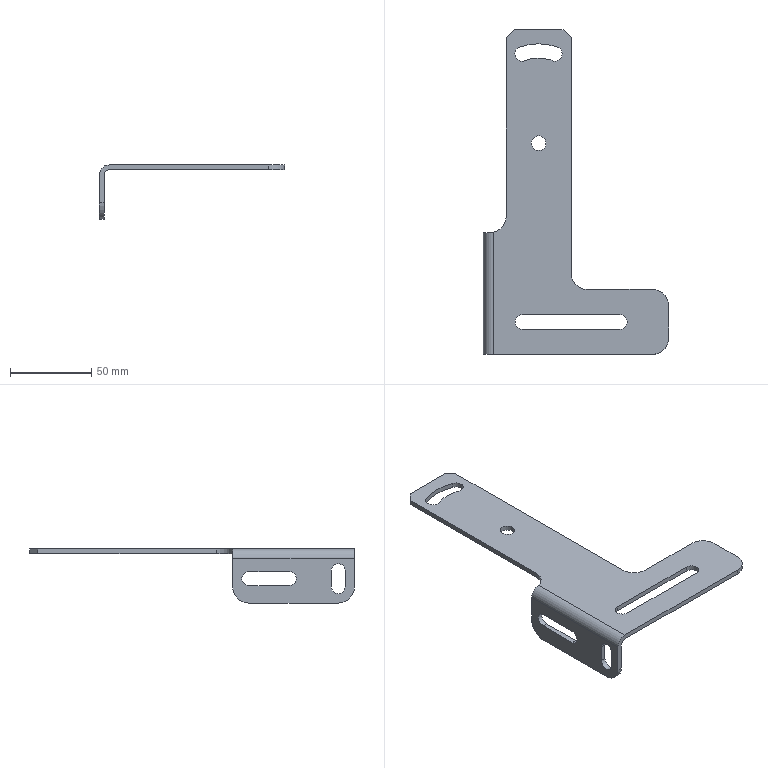Part | STEP file | S3 | 1 solid | 40 faces | box 114 x 200 x 33.288 mm | volume 36556 mm3 | plane 20 | cylinder 19 | spline 1 | commonest cylinder face diameters 20 x6 8.5 x4 9 x4 6 x1 9.209 x1 12 x1